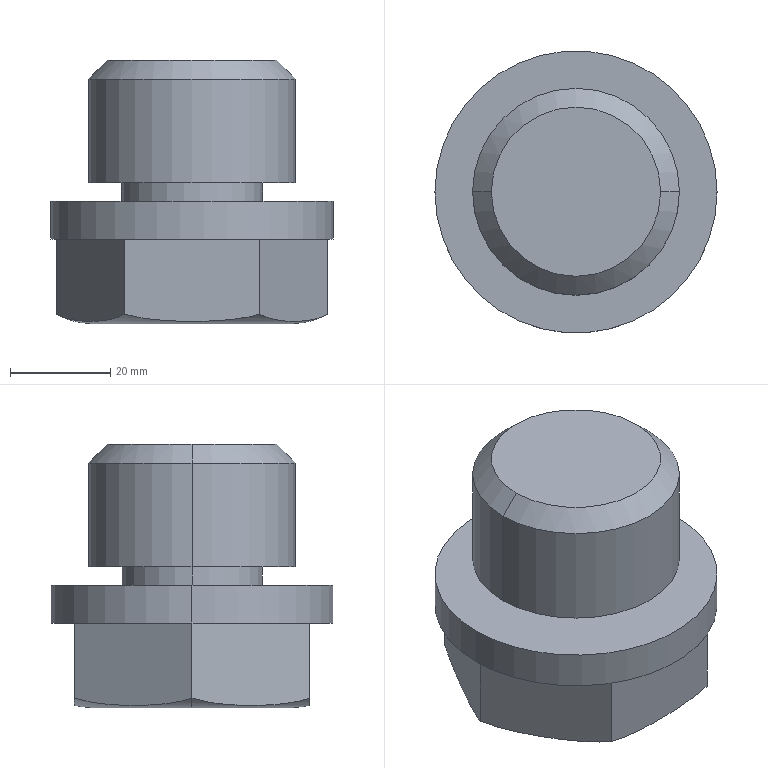Part | SolidWorks | features ICE 3, Chamfer 1, Extrusion 1, RevCut 1, Scale 1 | 1 solid | 21 faces | box 56.25 x 56.25 x 52.5 mm | volume 84582 mm3 | plane 11 | cylinder 6 | torus 2 | cone 2 | commonest cylinder face diameters 28.125 x2 41.25 x2 56.25 x2
STEP:
#1=CARTESIAN_POINT('',(20.033,-0.000002443,-10.956));
#2=VERTEX_POINT('',#1);
#3=CARTESIAN_POINT('',(-20.033,-0.000002443,-10.956));
#4=VERTEX_POINT('',#3);
#5=CARTESIAN_POINT('',(0.000000188,-0.000002443,-10.956));
#6=DIRECTION('',(0.,0.,1.));
#7=DIRECTION('',(1.,0.,0.));
#8=AXIS2_PLACEMENT_3D('',#5,#6,#7);
#9=CIRCLE('',#8,20.033);
#10=EDGE_CURVE('',#2,#4,#9,.T.);
#11=ORIENTED_EDGE('',*,*,#10,.T.);
#12=CARTESIAN_POINT('',(-27.063,-0.000002443,-9.081));
#13=VERTEX_POINT('',#12);
#14=CARTESIAN_POINT('',(-19.798,-0.000002443,4.042));
#15=DIRECTION('',(0.,1.,0.));
#16=DIRECTION('',(-1.,0.,0.));
#17=AXIS2_PLACEMENT_3D('',#14,#15,#16);
#18=CIRCLE('',#17,15.);
#19=EDGE_CURVE('',#4,#13,#18,.T.);
#20=ORIENTED_EDGE('',*,*,#19,.T.);
#21=CARTESIAN_POINT('',(-13.532,23.437,-9.081));
#22=VERTEX_POINT('',#21);
#23=CARTESIAN_POINT('',(-27.063,-0.000002443,-9.081));
#24=CARTESIAN_POINT('',(-26.508,0.9622,-9.389));
#25=CARTESIAN_POINT('',(-25.949,1.93,-9.624));
#26=CARTESIAN_POINT('',(-24.828,3.872,-9.995));
#27=CARTESIAN_POINT('',(-24.265,4.846,-10.131));
#28=CARTESIAN_POINT('',(-23.137,6.801,-10.334));
#29=CARTESIAN_POINT('',(-22.571,7.78,-10.402));
#30=CARTESIAN_POINT('',(-21.438,9.743,-10.489));
#31=CARTESIAN_POINT('',(-20.871,10.726,-10.509));
#32=CARTESIAN_POINT('',(-19.734,12.695,-10.51));
#33=CARTESIAN_POINT('',(-19.164,13.682,-10.49));
#34=CARTESIAN_POINT('',(-18.025,15.655,-10.402));
#35=CARTESIAN_POINT('',(-17.457,16.639,-10.334));
#36=CARTESIAN_POINT('',(-16.325,18.599,-10.13));
#37=CARTESIAN_POINT('',(-15.762,19.575,-9.994));
#38=CARTESIAN_POINT('',(-14.641,21.516,-9.622));
#39=CARTESIAN_POINT('',(-14.084,22.481,-9.387));
#40=CARTESIAN_POINT('',(-13.532,23.437,-9.081));
#41=B_SPLINE_CURVE_WITH_KNOTS('',3,(#23,#24,#25,#26,#27,#28,#29,#30,#31,#32,#33,#34,#35,#36,#37,#38,#39,#40),.UNSPECIFIED.,.F.,.F.,(4,2,2,2,2,2,2,2,4),(0.000000441,0.003399,0.006797,0.0102,0.01359,0.01699,0.02039,0.02379,0.02719),.UNSPECIFIED.);
#42=EDGE_CURVE('',#13,#22,#41,.T.);
#43=ORIENTED_EDGE('',*,*,#42,.T.);
#44=CARTESIAN_POINT('',(13.532,23.437,-9.081));
#45=VERTEX_POINT('',#44);
#46=CARTESIAN_POINT('',(-13.532,23.437,-9.081));
#47=CARTESIAN_POINT('',(-12.442,23.437,-9.383));
#48=CARTESIAN_POINT('',(-11.334,23.437,-9.618));
#49=CARTESIAN_POINT('',(-9.091,23.437,-9.991));
#50=CARTESIAN_POINT('',(-7.956,23.437,-10.129));
#51=CARTESIAN_POINT('',(-5.689,23.437,-10.334));
#52=CARTESIAN_POINT('',(-4.553,23.437,-10.401));
#53=CARTESIAN_POINT('',(-2.279,23.437,-10.489));
#54=CARTESIAN_POINT('',(-1.141,23.437,-10.51));
#55=CARTESIAN_POINT('',(1.138,23.437,-10.51));
#56=CARTESIAN_POINT('',(2.275,23.437,-10.489));
#57=CARTESIAN_POINT('',(4.545,23.437,-10.402));
#58=CARTESIAN_POINT('',(5.678,23.437,-10.334));
#59=CARTESIAN_POINT('',(7.938,23.437,-10.131));
#60=CARTESIAN_POINT('',(9.065,23.437,-9.995));
#61=CARTESIAN_POINT('',(10.748,23.437,-9.716));
#62=CARTESIAN_POINT('',(11.307,23.437,-9.61));
#63=CARTESIAN_POINT('',(12.424,23.437,-9.369));
#64=CARTESIAN_POINT('',(12.982,23.437,-9.233));
#65=CARTESIAN_POINT('',(13.532,23.437,-9.081));
#66=B_SPLINE_CURVE_WITH_KNOTS('',3,(#46,#47,#48,#49,#50,#51,#52,#53,#54,#55,#56,#57,#58,#59,#60,#61,#62,#63,#64,#65),.UNSPECIFIED.,.F.,.F.,(4,2,2,2,2,2,2,2,2,4),(0.1176,0.121,0.1244,0.1278,0.1312,0.1346,0.138,0.1414,0.1431,0.1448),.UNSPECIFIED.);
#67=EDGE_CURVE('',#22,#45,#66,.T.);
#68=ORIENTED_EDGE('',*,*,#67,.T.);
#69=CARTESIAN_POINT('',(27.063,-0.000002443,-9.081));
#70=VERTEX_POINT('',#69);
#71=CARTESIAN_POINT('',(13.532,23.437,-9.081));
#72=CARTESIAN_POINT('',(14.087,22.475,-9.389));
#73=CARTESIAN_POINT('',(14.646,21.508,-9.624));
#74=CARTESIAN_POINT('',(15.767,19.566,-9.995));
#75=CARTESIAN_POINT('',(16.33,18.591,-10.131));
#76=CARTESIAN_POINT('',(17.458,16.637,-10.334));
#77=CARTESIAN_POINT('',(18.024,15.657,-10.402));
#78=CARTESIAN_POINT('',(19.157,13.695,-10.489));
#79=CARTESIAN_POINT('',(19.724,12.712,-10.509));
#80=CARTESIAN_POINT('',(20.861,10.743,-10.51));
#81=CARTESIAN_POINT('',(21.431,9.756,-10.49));
#82=CARTESIAN_POINT('',(22.57,7.783,-10.402));
#83=CARTESIAN_POINT('',(23.138,6.799,-10.334));
#84=CARTESIAN_POINT('',(24.27,4.839,-10.13));
#85=CARTESIAN_POINT('',(24.833,3.863,-9.994));
#86=CARTESIAN_POINT('',(25.954,1.922,-9.622));
#87=CARTESIAN_POINT('',(26.511,0.9569,-9.387));
#88=CARTESIAN_POINT('',(27.063,-0.000002443,-9.081));
#89=B_SPLINE_CURVE_WITH_KNOTS('',3,(#71,#72,#73,#74,#75,#76,#77,#78,#79,#80,#81,#82,#83,#84,#85,#86,#87,#88),.UNSPECIFIED.,.F.,.F.,(4,2,2,2,2,2,2,2,4),(0.000000441,0.003399,0.006797,0.0102,0.01359,0.01699,0.02039,0.02379,0.02719),.UNSPECIFIED.);
#90=EDGE_CURVE('',#45,#70,#89,.T.);
#91=ORIENTED_EDGE('',*,*,#90,.T.);
#92=CARTESIAN_POINT('',(19.798,-0.000002443,4.042));
#93=DIRECTION('',(0.,-1.,0.));
#94=DIRECTION('',(0.,0.,-1.));
#95=AXIS2_PLACEMENT_3D('',#92,#93,#94);
#96=CIRCLE('',#95,15.);
#97=EDGE_CURVE('',#2,#70,#96,.T.);
#98=ORIENTED_EDGE('',*,*,#97,.F.);
#99=EDGE_LOOP('',(#11,#20,#43,#68,#91,#98));
#100=FACE_OUTER_BOUND('',#99,.T.);
#101=CARTESIAN_POINT('',(0.000000188,-0.000002443,4.042));
#102=DIRECTION('',(0.,0.,1.));
#103=DIRECTION('',(1.,0.,0.));
#104=AXIS2_PLACEMENT_3D('',#101,#102,#103);
#105=TOROIDAL_SURFACE('',#104,19.798,15.);
#106=ADVANCED_FACE('',(#100),#105,.T.);
#107=CARTESIAN_POINT('',(16.875,-0.000002443,41.544));
#108=VERTEX_POINT('',#107);
#109=CARTESIAN_POINT('',(-16.875,-0.000002443,41.544));
#110=VERTEX_POINT('',#109);
#111=CARTESIAN_POINT('',(0.000000188,-0.000002443,41.544));
#112=DIRECTION('',(0.,0.,1.));
#113=DIRECTION('',(1.,0.,0.));
#114=AXIS2_PLACEMENT_3D('',#111,#112,#113);
#115=CIRCLE('',#114,16.875);
#116=EDGE_CURVE('',#108,#110,#115,.T.);
#117=ORIENTED_EDGE('',*,*,#116,.F.);
#118=CARTESIAN_POINT('',(20.625,-0.000002443,37.794));
#119=VERTEX_POINT('',#118);
#120=CARTESIAN_POINT('',(16.875,-0.000002443,41.544));
#121=DIRECTION('',(0.7071,0.,-0.7071));
#122=VECTOR('',#121,1000.);
#123=LINE('',#120,#122);
#124=EDGE_CURVE('',#108,#119,#123,.T.);
#125=ORIENTED_EDGE('',*,*,#124,.T.);
#126=CARTESIAN_POINT('',(-20.625,-0.000002443,37.794));
#127=VERTEX_POINT('',#126);
#128=CARTESIAN_POINT('',(0.000000188,-0.000002443,37.794));
#129=DIRECTION('',(0.,0.,-1.));
#130=DIRECTION('',(1.,0.,0.));
#131=AXIS2_PLACEMENT_3D('',#128,#129,#130);
#132=CIRCLE('',#131,20.625);
#133=EDGE_CURVE('',#127,#119,#132,.T.);
#134=ORIENTED_EDGE('',*,*,#133,.F.);
#135=CARTESIAN_POINT('',(-16.875,-0.000002443,41.544));
#136=DIRECTION('',(-0.7071,0.,-0.7071));
#137=VECTOR('',#136,1000.);
#138=LINE('',#135,#137);
#139=EDGE_CURVE('',#110,#127,#138,.T.);
#140=ORIENTED_EDGE('',*,*,#139,.F.);
#141=EDGE_LOOP('',(#117,#125,#134,#140));
#142=FACE_OUTER_BOUND('',#141,.T.);
#143=CARTESIAN_POINT('',(0.000000188,-0.000002443,41.544));
#144=DIRECTION('',(0.,0.,-1.));
#145=DIRECTION('',(-1.,0.,0.));
#146=AXIS2_PLACEMENT_3D('',#143,#144,#145);
#147=CONICAL_SURFACE('',#146,16.875,0.7854);
#148=ADVANCED_FACE('',(#142),#147,.T.);
#149=ORIENTED_EDGE('',*,*,#133,.T.);
#150=CARTESIAN_POINT('',(20.625,-0.000002443,17.169));
#151=VERTEX_POINT('',#150);
#152=CARTESIAN_POINT('',(20.625,-0.000002443,41.544));
#153=DIRECTION('',(0.,0.,-1.));
#154=VECTOR('',#153,1000.);
#155=LINE('',#152,#154);
#156=EDGE_CURVE('',#119,#151,#155,.T.);
#157=ORIENTED_EDGE('',*,*,#156,.T.);
#158=CARTESIAN_POINT('',(-20.625,-0.000002443,17.169));
#159=VERTEX_POINT('',#158);
#160=CARTESIAN_POINT('',(0.000000188,-0.000002443,17.169));
#161=DIRECTION('',(0.,0.,1.));
#162=DIRECTION('',(1.,0.,0.));
#163=AXIS2_PLACEMENT_3D('',#160,#161,#162);
#164=CIRCLE('',#163,20.625);
#165=EDGE_CURVE('',#151,#159,#164,.T.);
#166=ORIENTED_EDGE('',*,*,#165,.T.);
#167=CARTESIAN_POINT('',(-20.625,-0.000002443,41.544));
#168=DIRECTION('',(0.,0.,-1.));
#169=VECTOR('',#168,1000.);
#170=LINE('',#167,#169);
#171=EDGE_CURVE('',#127,#159,#170,.T.);
#172=ORIENTED_EDGE('',*,*,#171,.F.);
#173=EDGE_LOOP('',(#149,#157,#166,#172));
#174=FACE_OUTER_BOUND('',#173,.T.);
#175=CARTESIAN_POINT('',(0.000000188,-0.000002443,41.544));
#176=DIRECTION('',(0.,0.,-1.));
#177=DIRECTION('',(-1.,0.,0.));
#178=AXIS2_PLACEMENT_3D('',#175,#176,#177);
#179=CYLINDRICAL_SURFACE('',#178,20.625);
#180=ADVANCED_FACE('',(#174),#179,.T.);
#181=CARTESIAN_POINT('',(14.063,-0.000002443,17.169));
#182=VERTEX_POINT('',#181);
#183=CARTESIAN_POINT('',(-14.062,-0.000002443,17.169));
#184=VERTEX_POINT('',#183);
#185=CARTESIAN_POINT('',(0.000000188,-0.000002443,17.169));
#186=DIRECTION('',(0.,0.,1.));
#187=DIRECTION('',(1.,0.,0.));
#188=AXIS2_PLACEMENT_3D('',#185,#186,#187);
#189=CIRCLE('',#188,14.062);
#190=EDGE_CURVE('',#182,#184,#189,.T.);
#191=ORIENTED_EDGE('',*,*,#190,.F.);
#192=CARTESIAN_POINT('',(14.063,-0.000002443,13.419));
#193=VERTEX_POINT('',#192);
#194=CARTESIAN_POINT('',(14.063,-0.000002443,17.169));
#195=DIRECTION('',(0.,0.,-1.));
#196=VECTOR('',#195,1000.);
#197=LINE('',#194,#196);
#198=EDGE_CURVE('',#182,#193,#197,.T.);
#199=ORIENTED_EDGE('',*,*,#198,.T.);
#200=CARTESIAN_POINT('',(-14.062,-0.000002443,13.419));
#201=VERTEX_POINT('',#200);
#202=CARTESIAN_POINT('',(0.000000188,-0.000002443,13.419));
#203=DIRECTION('',(0.,0.,1.));
#204=DIRECTION('',(1.,0.,0.));
#205=AXIS2_PLACEMENT_3D('',#202,#203,#204);
#206=CIRCLE('',#205,14.062);
#207=EDGE_CURVE('',#193,#201,#206,.T.);
#208=ORIENTED_EDGE('',*,*,#207,.T.);
#209=CARTESIAN_POINT('',(-14.062,-0.000002443,17.169));
#210=DIRECTION('',(0.,0.,-1.));
#211=VECTOR('',#210,1000.);
#212=LINE('',#209,#211);
#213=EDGE_CURVE('',#184,#201,#212,.T.);
#214=ORIENTED_EDGE('',*,*,#213,.F.);
#215=EDGE_LOOP('',(#191,#199,#208,#214));
#216=FACE_OUTER_BOUND('',#215,.T.);
#217=CARTESIAN_POINT('',(0.000000188,-0.000002443,17.169));
#218=DIRECTION('',(0.,0.,-1.));
#219=DIRECTION('',(-1.,0.,0.));
#220=AXIS2_PLACEMENT_3D('',#217,#218,#219);
#221=CYLINDRICAL_SURFACE('',#220,14.062);
#222=ADVANCED_FACE('',(#216),#221,.T.);
#223=CARTESIAN_POINT('',(28.125,-0.000002443,13.419));
#224=VERTEX_POINT('',#223);
#225=CARTESIAN_POINT('',(-28.125,-0.000002443,13.419));
#226=VERTEX_POINT('',#225);
#227=CARTESIAN_POINT('',(0.000000188,-0.000002443,13.419));
#228=DIRECTION('',(0.,0.,1.));
#229=DIRECTION('',(1.,0.,0.));
#230=AXIS2_PLACEMENT_3D('',#227,#228,#229);
#231=CIRCLE('',#230,28.125);
#232=EDGE_CURVE('',#224,#226,#231,.T.);
#233=ORIENTED_EDGE('',*,*,#232,.F.);
#234=CARTESIAN_POINT('',(28.125,-0.000002443,5.919));
#235=VERTEX_POINT('',#234);
#236=CARTESIAN_POINT('',(28.125,-0.000002443,13.419));
#237=DIRECTION('',(0.,0.,-1.));
#238=VECTOR('',#237,1000.);
#239=LINE('',#236,#238);
#240=EDGE_CURVE('',#224,#235,#239,.T.);
#241=ORIENTED_EDGE('',*,*,#240,.T.);
#242=CARTESIAN_POINT('',(-28.125,-0.000002443,5.919));
#243=VERTEX_POINT('',#242);
#244=CARTESIAN_POINT('',(0.000000188,-0.000002443,5.919));
#245=DIRECTION('',(0.,0.,1.));
#246=DIRECTION('',(1.,0.,0.));
#247=AXIS2_PLACEMENT_3D('',#244,#245,#246);
#248=CIRCLE('',#247,28.125);
#249=EDGE_CURVE('',#235,#243,#248,.T.);
#250=ORIENTED_EDGE('',*,*,#249,.T.);
#251=CARTESIAN_POINT('',(-28.125,-0.000002443,13.419));
#252=DIRECTION('',(0.,0.,-1.));
#253=VECTOR('',#252,1000.);
#254=LINE('',#251,#253);
#255=EDGE_CURVE('',#226,#243,#254,.T.);
#256=ORIENTED_EDGE('',*,*,#255,.F.);
#257=EDGE_LOOP('',(#233,#241,#250,#256));
#258=FACE_OUTER_BOUND('',#257,.T.);
#259=CARTESIAN_POINT('',(0.000000188,-0.000002443,13.419));
#260=DIRECTION('',(0.,0.,-1.));
#261=DIRECTION('',(-1.,0.,0.));
#262=AXIS2_PLACEMENT_3D('',#259,#260,#261);
#263=CYLINDRICAL_SURFACE('',#262,28.125);
#264=ADVANCED_FACE('',(#258),#263,.T.);
#265=CARTESIAN_POINT('',(13.532,-23.438,-9.081));
#266=VERTEX_POINT('',#265);
#267=CARTESIAN_POINT('',(27.063,-0.000002443,-9.081));
#268=CARTESIAN_POINT('',(26.508,-0.9622,-9.389));
#269=CARTESIAN_POINT('',(25.949,-1.93,-9.624));
#270=CARTESIAN_POINT('',(24.828,-3.872,-9.995));
#271=CARTESIAN_POINT('',(24.265,-4.846,-10.131));
#272=CARTESIAN_POINT('',(23.137,-6.801,-10.334));
#273=CARTESIAN_POINT('',(22.571,-7.78,-10.402));
#274=CARTESIAN_POINT('',(21.438,-9.743,-10.489));
#275=CARTESIAN_POINT('',(20.871,-10.726,-10.509));
#276=CARTESIAN_POINT('',(19.734,-12.695,-10.51));
#277=CARTESIAN_POINT('',(19.164,-13.682,-10.49));
#278=CARTESIAN_POINT('',(18.025,-15.655,-10.402));
#279=CARTESIAN_POINT('',(17.457,-16.639,-10.334));
#280=CARTESIAN_POINT('',(16.325,-18.599,-10.13));
#281=CARTESIAN_POINT('',(15.762,-19.575,-9.994));
#282=CARTESIAN_POINT('',(14.641,-21.516,-9.622));
#283=CARTESIAN_POINT('',(14.084,-22.481,-9.387));
#284=CARTESIAN_POINT('',(13.532,-23.438,-9.081));
#285=B_SPLINE_CURVE_WITH_KNOTS('',3,(#267,#268,#269,#270,#271,#272,#273,#274,#275,#276,#277,#278,#279,#280,#281,#282,#283,#284),.UNSPECIFIED.,.F.,.F.,(4,2,2,2,2,2,2,2,4),(0.000000441,0.003399,0.006797,0.0102,0.01359,0.01699,0.02039,0.02379,0.02719),.UNSPECIFIED.);
#286=EDGE_CURVE('',#70,#266,#285,.T.);
#287=ORIENTED_EDGE('',*,*,#286,.F.);
#288=CARTESIAN_POINT('',(27.063,-0.000002443,5.919));
#289=VERTEX_POINT('',#288);
#290=CARTESIAN_POINT('',(27.063,-0.000002443,5.919));
#291=DIRECTION('',(0.,0.,-1.));
#292=VECTOR('',#291,1000.);
#293=LINE('',#290,#292);
#294=EDGE_CURVE('',#289,#70,#293,.T.);
#295=ORIENTED_EDGE('',*,*,#294,.F.);
#296=CARTESIAN_POINT('',(13.532,-23.438,5.919));
#297=VERTEX_POINT('',#296);
#298=CARTESIAN_POINT('',(13.532,-23.438,5.919));
#299=DIRECTION('',(0.5,0.866,0.));
#300=VECTOR('',#299,1000.);
#301=LINE('',#298,#300);
#302=EDGE_CURVE('',#297,#289,#301,.T.);
#303=ORIENTED_EDGE('',*,*,#302,.F.);
#304=CARTESIAN_POINT('',(13.532,-23.438,5.919));
#305=DIRECTION('',(0.,0.,-1.));
#306=VECTOR('',#305,1000.);
#307=LINE('',#304,#306);
#308=EDGE_CURVE('',#297,#266,#307,.T.);
#309=ORIENTED_EDGE('',*,*,#308,.T.);
#310=EDGE_LOOP('',(#287,#295,#303,#309));
#311=FACE_OUTER_BOUND('',#310,.T.);
#312=CARTESIAN_POINT('',(13.532,-23.438,5.919));
#313=DIRECTION('',(-0.866,0.5,0.));
#314=DIRECTION('',(-0.5,-0.866,0.));
#315=AXIS2_PLACEMENT_3D('',#312,#313,#314);
#316=PLANE('',#315);
#317=ADVANCED_FACE('',(#311),#316,.F.);
#318=ORIENTED_EDGE('',*,*,#90,.F.);
#319=CARTESIAN_POINT('',(13.532,23.437,5.919));
#320=VERTEX_POINT('',#319);
#321=CARTESIAN_POINT('',(13.532,23.437,5.919));
#322=DIRECTION('',(0.,0.,-1.));
#323=VECTOR('',#322,1000.);
#324=LINE('',#321,#323);
#325=EDGE_CURVE('',#320,#45,#324,.T.);
#326=ORIENTED_EDGE('',*,*,#325,.F.);
#327=CARTESIAN_POINT('',(27.063,-0.000002443,5.919));
#328=DIRECTION('',(-0.5,0.866,0.));
#329=VECTOR('',#328,1000.);
#330=LINE('',#327,#329);
#331=EDGE_CURVE('',#289,#320,#330,.T.);
#332=ORIENTED_EDGE('',*,*,#331,.F.);
#333=ORIENTED_EDGE('',*,*,#294,.T.);
#334=EDGE_LOOP('',(#318,#326,#332,#333));
#335=FACE_OUTER_BOUND('',#334,.T.);
#336=CARTESIAN_POINT('',(27.063,-0.000002443,5.919));
#337=DIRECTION('',(-0.866,-0.5,0.));
#338=DIRECTION('',(0.5,-0.866,0.));
#339=AXIS2_PLACEMENT_3D('',#336,#337,#338);
#340=PLANE('',#339);
#341=ADVANCED_FACE('',(#335),#340,.F.);
#342=ORIENTED_EDGE('',*,*,#67,.F.);
#343=CARTESIAN_POINT('',(-13.532,23.437,5.919));
#344=VERTEX_POINT('',#343);
#345=CARTESIAN_POINT('',(-13.532,23.437,5.919));
#346=DIRECTION('',(0.,0.,-1.));
#347=VECTOR('',#346,1000.);
#348=LINE('',#345,#347);
#349=EDGE_CURVE('',#344,#22,#348,.T.);
#350=ORIENTED_EDGE('',*,*,#349,.F.);
#351=CARTESIAN_POINT('',(13.532,23.437,5.919));
#352=DIRECTION('',(-1.,0.,0.));
#353=VECTOR('',#352,1000.);
#354=LINE('',#351,#353);
#355=EDGE_CURVE('',#320,#344,#354,.T.);
#356=ORIENTED_EDGE('',*,*,#355,.F.);
#357=ORIENTED_EDGE('',*,*,#325,.T.);
#358=EDGE_LOOP('',(#342,#350,#356,#357));
#359=FACE_OUTER_BOUND('',#358,.T.);
#360=CARTESIAN_POINT('',(13.532,23.437,5.919));
#361=DIRECTION('',(0.,-1.,0.));
#362=DIRECTION('',(0.,0.,-1.));
#363=AXIS2_PLACEMENT_3D('',#360,#361,#362);
#364=PLANE('',#363);
#365=ADVANCED_FACE('',(#359),#364,.F.);
#366=ORIENTED_EDGE('',*,*,#42,.F.);
#367=CARTESIAN_POINT('',(-27.063,-0.000002443,5.919));
#368=VERTEX_POINT('',#367);
#369=CARTESIAN_POINT('',(-27.063,-0.000002443,5.919));
#370=DIRECTION('',(0.,0.,-1.));
#371=VECTOR('',#370,1000.);
#372=LINE('',#369,#371);
#373=EDGE_CURVE('',#368,#13,#372,.T.);
#374=ORIENTED_EDGE('',*,*,#373,.F.);
#375=CARTESIAN_POINT('',(-13.532,23.437,5.919));
#376=DIRECTION('',(-0.5,-0.866,0.));
#377=VECTOR('',#376,1000.);
#378=LINE('',#375,#377);
#379=EDGE_CURVE('',#344,#368,#378,.T.);
#380=ORIENTED_EDGE('',*,*,#379,.F.);
#381=ORIENTED_EDGE('',*,*,#349,.T.);
#382=EDGE_LOOP('',(#366,#374,#380,#381));
#383=FACE_OUTER_BOUND('',#382,.T.);
#384=CARTESIAN_POINT('',(-13.532,23.437,5.919));
#385=DIRECTION('',(0.866,-0.5,0.));
#386=DIRECTION('',(0.5,0.866,0.));
#387=AXIS2_PLACEMENT_3D('',#384,#385,#386);
#388=PLANE('',#387);
#389=ADVANCED_FACE('',(#383),#388,.F.);
#390=CARTESIAN_POINT('',(-13.532,-23.438,-9.081));
#391=VERTEX_POINT('',#390);
#392=CARTESIAN_POINT('',(-13.532,-23.438,-9.081));
#393=CARTESIAN_POINT('',(-14.087,-22.475,-9.389));
#394=CARTESIAN_POINT('',(-14.646,-21.508,-9.624));
#395=CARTESIAN_POINT('',(-15.767,-19.566,-9.995));
#396=CARTESIAN_POINT('',(-16.33,-18.591,-10.131));
#397=CARTESIAN_POINT('',(-17.458,-16.637,-10.334));
#398=CARTESIAN_POINT('',(-18.024,-15.657,-10.402));
#399=CARTESIAN_POINT('',(-19.157,-13.695,-10.489));
#400=CARTESIAN_POINT('',(-19.724,-12.712,-10.509));
#401=CARTESIAN_POINT('',(-20.861,-10.743,-10.51));
#402=CARTESIAN_POINT('',(-21.431,-9.756,-10.49));
#403=CARTESIAN_POINT('',(-22.57,-7.783,-10.402));
#404=CARTESIAN_POINT('',(-23.138,-6.799,-10.334));
#405=CARTESIAN_POINT('',(-24.27,-4.839,-10.13));
#406=CARTESIAN_POINT('',(-24.833,-3.863,-9.994));
#407=CARTESIAN_POINT('',(-25.954,-1.922,-9.622));
#408=CARTESIAN_POINT('',(-26.511,-0.9569,-9.387));
#409=CARTESIAN_POINT('',(-27.063,-0.000002443,-9.081));
#410=B_SPLINE_CURVE_WITH_KNOTS('',3,(#392,#393,#394,#395,#396,#397,#398,#399,#400,#401,#402,#403,#404,#405,#406,#407,#408,#409),.UNSPECIFIED.,.F.,.F.,(4,2,2,2,2,2,2,2,4),(0.000000441,0.003399,0.006797,0.0102,0.01359,0.01699,0.02039,0.02379,0.02719),.UNSPECIFIED.);
#411=EDGE_CURVE('',#391,#13,#410,.T.);
#412=ORIENTED_EDGE('',*,*,#411,.F.);
#413=CARTESIAN_POINT('',(-13.532,-23.438,5.919));
#414=VERTEX_POINT('',#413);
#415=CARTESIAN_POINT('',(-13.532,-23.438,5.919));
#416=DIRECTION('',(0.,0.,-1.));
#417=VECTOR('',#416,1000.);
#418=LINE('',#415,#417);
#419=EDGE_CURVE('',#414,#391,#418,.T.);
#420=ORIENTED_EDGE('',*,*,#419,.F.);
#421=CARTESIAN_POINT('',(-27.063,-0.000002443,5.919));
#422=DIRECTION('',(0.5,-0.866,0.));
#423=VECTOR('',#422,1000.);
#424=LINE('',#421,#423);
#425=EDGE_CURVE('',#368,#414,#424,.T.);
#426=ORIENTED_EDGE('',*,*,#425,.F.);
#427=ORIENTED_EDGE('',*,*,#373,.T.);
#428=EDGE_LOOP('',(#412,#420,#426,#427));
#429=FACE_OUTER_BOUND('',#428,.T.);
#430=CARTESIAN_POINT('',(-27.063,-0.000002443,5.919));
#431=DIRECTION('',(0.866,0.5,0.));
#432=DIRECTION('',(-0.5,0.866,0.));
#433=AXIS2_PLACEMENT_3D('',#430,#431,#432);
#434=PLANE('',#433);
#435=ADVANCED_FACE('',(#429),#434,.F.);
#436=CARTESIAN_POINT('',(13.532,-23.438,-9.081));
#437=CARTESIAN_POINT('',(12.442,-23.438,-9.383));
#438=CARTESIAN_POINT('',(11.334,-23.438,-9.618));
#439=CARTESIAN_POINT('',(9.091,-23.438,-9.991));
#440=CARTESIAN_POINT('',(7.956,-23.438,-10.129));
#441=CARTESIAN_POINT('',(5.689,-23.438,-10.334));
#442=CARTESIAN_POINT('',(4.553,-23.438,-10.401));
#443=CARTESIAN_POINT('',(2.279,-23.438,-10.489));
#444=CARTESIAN_POINT('',(1.141,-23.438,-10.51));
#445=CARTESIAN_POINT('',(-1.138,-23.438,-10.51));
#446=CARTESIAN_POINT('',(-2.275,-23.438,-10.489));
#447=CARTESIAN_POINT('',(-4.545,-23.438,-10.402));
#448=CARTESIAN_POINT('',(-5.678,-23.438,-10.334));
#449=CARTESIAN_POINT('',(-7.938,-23.438,-10.131));
#450=CARTESIAN_POINT('',(-9.065,-23.438,-9.995));
#451=CARTESIAN_POINT('',(-10.748,-23.438,-9.716));
#452=CARTESIAN_POINT('',(-11.307,-23.438,-9.61));
#453=CARTESIAN_POINT('',(-12.424,-23.438,-9.369));
#454=CARTESIAN_POINT('',(-12.982,-23.438,-9.233));
#455=CARTESIAN_POINT('',(-13.532,-23.438,-9.081));
#456=B_SPLINE_CURVE_WITH_KNOTS('',3,(#436,#437,#438,#439,#440,#441,#442,#443,#444,#445,#446,#447,#448,#449,#450,#451,#452,#453,#454,#455),.UNSPECIFIED.,.F.,.F.,(4,2,2,2,2,2,2,2,2,4),(0.1176,0.121,0.1244,0.1278,0.1312,0.1346,0.138,0.1414,0.1431,0.1448),.UNSPECIFIED.);
#457=EDGE_CURVE('',#266,#391,#456,.T.);
#458=ORIENTED_EDGE('',*,*,#457,.F.);
#459=ORIENTED_EDGE('',*,*,#308,.F.);
#460=CARTESIAN_POINT('',(-13.532,-23.438,5.919));
#461=DIRECTION('',(1.,0.,0.));
#462=VECTOR('',#461,1000.);
#463=LINE('',#460,#462);
#464=EDGE_CURVE('',#414,#297,#463,.T.);
#465=ORIENTED_EDGE('',*,*,#464,.F.);
#466=ORIENTED_EDGE('',*,*,#419,.T.);
#467=EDGE_LOOP('',(#458,#459,#465,#466));
#468=FACE_OUTER_BOUND('',#467,.T.);
#469=CARTESIAN_POINT('',(-13.532,-23.438,5.919));
#470=DIRECTION('',(0.,1.,0.));
#471=DIRECTION('',(0.,0.,1.));
#472=AXIS2_PLACEMENT_3D('',#469,#470,#471);
#473=PLANE('',#472);
#474=ADVANCED_FACE('',(#468),#473,.F.);
#475=CARTESIAN_POINT('',(0.000000188,-0.000002443,13.419));
#476=DIRECTION('',(0.,0.,1.));
#477=DIRECTION('',(1.,0.,0.));
#478=AXIS2_PLACEMENT_3D('',#475,#476,#477);
#479=CIRCLE('',#478,28.125);
#480=EDGE_CURVE('',#226,#224,#479,.T.);
#481=ORIENTED_EDGE('',*,*,#480,.T.);
#482=ORIENTED_EDGE('',*,*,#232,.T.);
#483=EDGE_LOOP('',(#481,#482));
#484=FACE_OUTER_BOUND('',#483,.T.);
#485=CARTESIAN_POINT('',(0.000000188,-0.000002443,13.419));
#486=DIRECTION('',(0.,0.,1.));
#487=DIRECTION('',(1.,0.,0.));
#488=AXIS2_PLACEMENT_3D('',#485,#486,#487);
#489=CIRCLE('',#488,14.062);
#490=EDGE_CURVE('',#201,#193,#489,.T.);
#491=ORIENTED_EDGE('',*,*,#490,.F.);
#492=ORIENTED_EDGE('',*,*,#207,.F.);
#493=EDGE_LOOP('',(#491,#492));
#494=FACE_BOUND('',#493,.T.);
#495=CARTESIAN_POINT('',(0.000000188,-0.000002443,13.419));
#496=DIRECTION('',(0.,0.,1.));
#497=DIRECTION('',(1.,0.,0.));
#498=AXIS2_PLACEMENT_3D('',#495,#496,#497);
#499=PLANE('',#498);
#500=ADVANCED_FACE('',(#484,#494),#499,.T.);
#501=CARTESIAN_POINT('',(0.000000188,-0.000002443,5.919));
#502=DIRECTION('',(0.,0.,1.));
#503=DIRECTION('',(1.,0.,0.));
#504=AXIS2_PLACEMENT_3D('',#501,#502,#503);
#505=CIRCLE('',#504,28.125);
#506=EDGE_CURVE('',#243,#235,#505,.T.);
#507=ORIENTED_EDGE('',*,*,#506,.F.);
#508=ORIENTED_EDGE('',*,*,#249,.F.);
#509=EDGE_LOOP('',(#507,#508));
#510=FACE_OUTER_BOUND('',#509,.T.);
#511=ORIENTED_EDGE('',*,*,#464,.T.);
#512=ORIENTED_EDGE('',*,*,#302,.T.);
#513=ORIENTED_EDGE('',*,*,#331,.T.);
#514=ORIENTED_EDGE('',*,*,#355,.T.);
#515=ORIENTED_EDGE('',*,*,#379,.T.);
#516=ORIENTED_EDGE('',*,*,#425,.T.);
#517=EDGE_LOOP('',(#511,#512,#513,#514,#515,#516));
#518=FACE_BOUND('',#517,.T.);
#519=CARTESIAN_POINT('',(0.000000188,-0.000002443,5.919));
#520=DIRECTION('',(0.,0.,1.));
#521=DIRECTION('',(1.,0.,0.));
#522=AXIS2_PLACEMENT_3D('',#519,#520,#521);
#523=PLANE('',#522);
#524=ADVANCED_FACE('',(#510,#518),#523,.F.);
#525=ORIENTED_EDGE('',*,*,#240,.F.);
#526=ORIENTED_EDGE('',*,*,#480,.F.);
#527=ORIENTED_EDGE('',*,*,#255,.T.);
#528=ORIENTED_EDGE('',*,*,#506,.T.);
#529=EDGE_LOOP('',(#525,#526,#527,#528));
#530=FACE_OUTER_BOUND('',#529,.T.);
#531=CARTESIAN_POINT('',(0.000000188,-0.000002443,13.419));
#532=DIRECTION('',(0.,0.,-1.));
#533=DIRECTION('',(-1.,0.,0.));
#534=AXIS2_PLACEMENT_3D('',#531,#532,#533);
#535=CYLINDRICAL_SURFACE('',#534,28.125);
#536=ADVANCED_FACE('',(#530),#535,.T.);
#537=ORIENTED_EDGE('',*,*,#198,.F.);
#538=CARTESIAN_POINT('',(0.000000188,-0.000002443,17.169));
#539=DIRECTION('',(0.,0.,1.));
#540=DIRECTION('',(1.,0.,0.));
#541=AXIS2_PLACEMENT_3D('',#538,#539,#540);
#542=CIRCLE('',#541,14.062);
#543=EDGE_CURVE('',#184,#182,#542,.T.);
#544=ORIENTED_EDGE('',*,*,#543,.F.);
#545=ORIENTED_EDGE('',*,*,#213,.T.);
#546=ORIENTED_EDGE('',*,*,#490,.T.);
#547=EDGE_LOOP('',(#537,#544,#545,#546));
#548=FACE_OUTER_BOUND('',#547,.T.);
#549=CARTESIAN_POINT('',(0.000000188,-0.000002443,17.169));
#550=DIRECTION('',(0.,0.,-1.));
#551=DIRECTION('',(-1.,0.,0.));
#552=AXIS2_PLACEMENT_3D('',#549,#550,#551);
#553=CYLINDRICAL_SURFACE('',#552,14.062);
#554=ADVANCED_FACE('',(#548),#553,.T.);
#555=CARTESIAN_POINT('',(0.000000188,-0.000002443,17.169));
#556=DIRECTION('',(0.,0.,1.));
#557=DIRECTION('',(1.,0.,0.));
#558=AXIS2_PLACEMENT_3D('',#555,#556,#557);
#559=CIRCLE('',#558,20.625);
#560=EDGE_CURVE('',#159,#151,#559,.T.);
#561=ORIENTED_EDGE('',*,*,#560,.F.);
#562=ORIENTED_EDGE('',*,*,#165,.F.);
#563=EDGE_LOOP('',(#561,#562));
#564=FACE_OUTER_BOUND('',#563,.T.);
#565=ORIENTED_EDGE('',*,*,#543,.T.);
#566=ORIENTED_EDGE('',*,*,#190,.T.);
#567=EDGE_LOOP('',(#565,#566));
#568=FACE_BOUND('',#567,.T.);
#569=CARTESIAN_POINT('',(0.000000188,-0.000002443,17.169));
#570=DIRECTION('',(0.,0.,1.));
#571=DIRECTION('',(1.,0.,0.));
#572=AXIS2_PLACEMENT_3D('',#569,#570,#571);
#573=PLANE('',#572);
#574=ADVANCED_FACE('',(#564,#568),#573,.F.);
#575=ORIENTED_EDGE('',*,*,#156,.F.);
#576=CARTESIAN_POINT('',(0.000000188,-0.000002443,37.794));
#577=DIRECTION('',(0.,0.,-1.));
#578=DIRECTION('',(1.,0.,0.));
#579=AXIS2_PLACEMENT_3D('',#576,#577,#578);
#580=CIRCLE('',#579,20.625);
#581=EDGE_CURVE('',#119,#127,#580,.T.);
#582=ORIENTED_EDGE('',*,*,#581,.T.);
#583=ORIENTED_EDGE('',*,*,#171,.T.);
#584=ORIENTED_EDGE('',*,*,#560,.T.);
#585=EDGE_LOOP('',(#575,#582,#583,#584));
#586=FACE_OUTER_BOUND('',#585,.T.);
#587=CARTESIAN_POINT('',(0.000000188,-0.000002443,41.544));
#588=DIRECTION('',(0.,0.,-1.));
#589=DIRECTION('',(-1.,0.,0.));
#590=AXIS2_PLACEMENT_3D('',#587,#588,#589);
#591=CYLINDRICAL_SURFACE('',#590,20.625);
#592=ADVANCED_FACE('',(#586),#591,.T.);
#593=CARTESIAN_POINT('',(0.000000188,-0.000002443,41.544));
#594=DIRECTION('',(0.,0.,1.));
#595=DIRECTION('',(1.,0.,0.));
#596=AXIS2_PLACEMENT_3D('',#593,#594,#595);
#597=CIRCLE('',#596,16.875);
#598=EDGE_CURVE('',#110,#108,#597,.T.);
#599=ORIENTED_EDGE('',*,*,#598,.T.);
#600=ORIENTED_EDGE('',*,*,#116,.T.);
#601=EDGE_LOOP('',(#599,#600));
#602=FACE_OUTER_BOUND('',#601,.T.);
#603=CARTESIAN_POINT('',(0.000000188,-0.000002443,41.544));
#604=DIRECTION('',(0.,0.,1.));
#605=DIRECTION('',(1.,0.,0.));
#606=AXIS2_PLACEMENT_3D('',#603,#604,#605);
#607=PLANE('',#606);
#608=ADVANCED_FACE('',(#602),#607,.T.);
#609=ORIENTED_EDGE('',*,*,#124,.F.);
#610=ORIENTED_EDGE('',*,*,#598,.F.);
#611=ORIENTED_EDGE('',*,*,#139,.T.);
#612=ORIENTED_EDGE('',*,*,#581,.F.);
#613=EDGE_LOOP('',(#609,#610,#611,#612));
#614=FACE_OUTER_BOUND('',#613,.T.);
#615=CARTESIAN_POINT('',(0.000000188,-0.000002443,41.544));
#616=DIRECTION('',(0.,0.,-1.));
#617=DIRECTION('',(-1.,0.,0.));
#618=AXIS2_PLACEMENT_3D('',#615,#616,#617);
#619=CONICAL_SURFACE('',#618,16.875,0.7854);
#620=ADVANCED_FACE('',(#614),#619,.T.);
#621=ORIENTED_EDGE('',*,*,#19,.F.);
#622=CARTESIAN_POINT('',(0.000000188,-0.000002443,-10.956));
#623=DIRECTION('',(0.,0.,1.));
#624=DIRECTION('',(1.,0.,0.));
#625=AXIS2_PLACEMENT_3D('',#622,#623,#624);
#626=CIRCLE('',#625,20.033);
#627=EDGE_CURVE('',#4,#2,#626,.T.);
#628=ORIENTED_EDGE('',*,*,#627,.T.);
#629=ORIENTED_EDGE('',*,*,#97,.T.);
#630=ORIENTED_EDGE('',*,*,#286,.T.);
#631=ORIENTED_EDGE('',*,*,#457,.T.);
#632=ORIENTED_EDGE('',*,*,#411,.T.);
#633=EDGE_LOOP('',(#621,#628,#629,#630,#631,#632));
#634=FACE_OUTER_BOUND('',#633,.T.);
#635=CARTESIAN_POINT('',(0.000000188,-0.000002443,4.042));
#636=DIRECTION('',(0.,0.,1.));
#637=DIRECTION('',(1.,0.,0.));
#638=AXIS2_PLACEMENT_3D('',#635,#636,#637);
#639=TOROIDAL_SURFACE('',#638,19.798,15.);
#640=ADVANCED_FACE('',(#634),#639,.T.);
#641=ORIENTED_EDGE('',*,*,#10,.F.);
#642=ORIENTED_EDGE('',*,*,#627,.F.);
#643=EDGE_LOOP('',(#641,#642));
#644=FACE_OUTER_BOUND('',#643,.T.);
#645=CARTESIAN_POINT('',(0.000000188,-0.000002443,-10.956));
#646=DIRECTION('',(0.,0.,1.));
#647=DIRECTION('',(1.,0.,0.));
#648=AXIS2_PLACEMENT_3D('',#645,#646,#647);
#649=PLANE('',#648);
#650=ADVANCED_FACE('',(#644),#649,.F.);
#651=CLOSED_SHELL('',(#106,#148,#180,#222,#264,#317,#341,#365,#389,#435,#474,#500,#524,#536,#554,#574,#592,#608,#620,#640,#650));
#652=MANIFOLD_SOLID_BREP('',#651);
#653=CARTESIAN_POINT('',(0.,0.,0.));
#654=DIRECTION('',(0.,0.,1.));
#655=DIRECTION('',(1.,0.,0.));
#656=AXIS2_PLACEMENT_3D('',#653,#654,#655);
#657=(LENGTH_UNIT()NAMED_UNIT(*)SI_UNIT(.MILLI.,.METRE.));
#658=UNCERTAINTY_MEASURE_WITH_UNIT(LENGTH_MEASURE(0.00001),#657,'','');
#659=(NAMED_UNIT(*)PLANE_ANGLE_UNIT()SI_UNIT($,.RADIAN.));
#660=(NAMED_UNIT(*)SI_UNIT($,.STERADIAN.)SOLID_ANGLE_UNIT());
#661=(GEOMETRIC_REPRESENTATION_CONTEXT(3)GLOBAL_UNCERTAINTY_ASSIGNED_CONTEXT((#658))GLOBAL_UNIT_ASSIGNED_CONTEXT((#657,#659,#660))REPRESENTATION_CONTEXT('',''));
#662=ADVANCED_BREP_SHAPE_REPRESENTATION('',(#652,#656),#661);